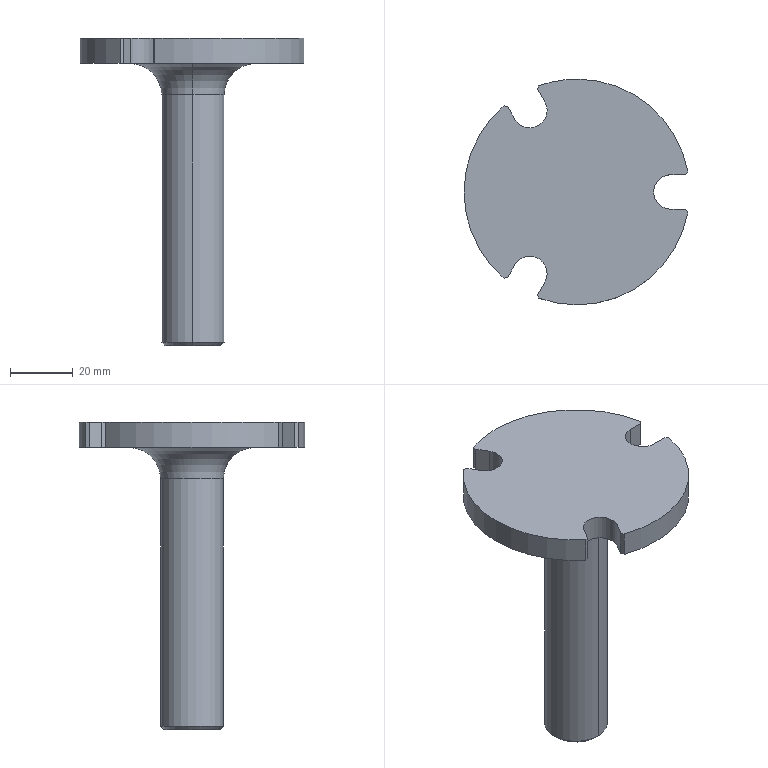NC program | NX | posted with a generic post | part box 71.434 x 72 x 98 mm
Lines 1 to 922 of 11060:
N10 G17 G21 G94 G90
(ZLEVEL_PROFILE_COPY_1 , TOOL : D6C)
N12 T06 M6
N14 G54
N16 G17 G0 G90 X-25.933 Y32.567 S5000 M3
N18 G43 Z30. H6
N20 Z-0.05
N22 G94 G1 X-25.748 Y31.712 F1800.
N24 G3 X-25.344 Y31.268 R0.6
N26 G1 X-22.161 Y30.416
N28 X-20.99 Y30.102
N30 G2 X-19.162 Y28.7 R3.01
N32 G1 X-16.874 Y24.736
N34 G3 X-13.472 Y23.824 R2.49
N36 X-12.561 Y27.226 R2.49
N38 G1 X-14.849 Y31.19
N40 G2 X-15.074 Y33.718 R3.01
N42 G1 X-15.079 Y33.731
N44 X-15.031 Y33.919
N46 X-14.836 Y34.644
N48 X-14.763 Y34.88
N50 X-14.77 Y34.888
N52 X-13.984 Y37.824
N54 G3 X-14.139 Y38.404 R0.6
N56 G1 X-14.782 Y39.046
N58 G0 X-26.004 Y32.57 Z-0.1
N60 G1 X-25.769 Y31.692
N62 G3 X-25.344 Y31.268 R0.6
N64 G1 X-22.161 Y30.416
N66 X-20.99 Y30.102
N68 G2 X-19.162 Y28.7 R3.01
N70 G1 X-16.874 Y24.736
N72 G3 X-13.472 Y23.824 R2.49
N74 X-12.561 Y27.226 R2.49
N76 G1 X-14.849 Y31.19
N78 G2 X-15.074 Y33.718 R3.01
N80 G1 X-15.079 Y33.731
N82 X-15.031 Y33.919
N84 X-14.836 Y34.644
N86 X-14.763 Y34.88
N88 X-14.77 Y34.888
N90 X-13.984 Y37.824
N92 G3 X-14.139 Y38.404 R0.6
N94 G1 X-14.782 Y39.046
N96 G0 X-26.004 Y32.57 Z-0.15
N98 G1 X-25.769 Y31.692
N100 G3 X-25.344 Y31.268 R0.6
N102 G1 X-22.161 Y30.416
N104 X-20.99 Y30.102
N106 G2 X-19.162 Y28.7 R3.01
N108 G1 X-16.874 Y24.736
N110 G3 X-13.472 Y23.824 R2.49
N112 X-12.561 Y27.226 R2.49
N114 G1 X-14.849 Y31.19
N116 G2 X-15.074 Y33.718 R3.01
N118 G1 X-15.079 Y33.731
N120 X-15.031 Y33.919
N122 X-14.836 Y34.644
N124 X-14.763 Y34.88
N126 X-14.77 Y34.888
N128 X-13.984 Y37.824
N130 G3 X-14.139 Y38.404 R0.6
N132 G1 X-14.782 Y39.046
N134 G0 X-26.004 Y32.57 Z-0.2
N136 G1 X-25.769 Y31.692
N138 G3 X-25.344 Y31.268 R0.6
N140 G1 X-22.161 Y30.416
N142 X-20.99 Y30.102
N144 G2 X-19.162 Y28.7 R3.01
N146 G1 X-16.874 Y24.736
N148 G3 X-13.472 Y23.824 R2.49
N150 X-12.561 Y27.226 R2.49
N152 G1 X-14.849 Y31.19
N154 G2 X-15.074 Y33.718 R3.01
N156 G1 X-15.079 Y33.731
N158 X-15.031 Y33.919
N160 X-14.836 Y34.644
N162 X-14.763 Y34.88
N164 X-14.77 Y34.888
N166 X-13.984 Y37.824
N168 G3 X-14.139 Y38.404 R0.6
N170 G1 X-14.782 Y39.046
N172 G0 X-26.004 Y32.57 Z-0.25
N174 G1 X-25.769 Y31.692
N176 G3 X-25.344 Y31.268 R0.6
N178 G1 X-22.161 Y30.416
N180 X-20.99 Y30.102
N182 G2 X-19.162 Y28.7 R3.01
N184 G1 X-16.874 Y24.736
N186 G3 X-13.472 Y23.824 R2.49
N188 X-12.561 Y27.226 R2.49
N190 G1 X-14.849 Y31.19
N192 G2 X-15.074 Y33.718 R3.01
N194 G1 X-15.079 Y33.731
N196 X-15.031 Y33.919
N198 X-14.836 Y34.645
N200 X-14.763 Y34.88
N202 X-14.77 Y34.888
N204 X-13.984 Y37.824
N206 G3 X-14.139 Y38.404 R0.6
N208 G1 X-14.782 Y39.046
N210 G0 X-26.004 Y32.57 Z-0.3
N212 G1 X-25.769 Y31.692
N214 G3 X-25.344 Y31.268 R0.6
N216 G1 X-22.161 Y30.416
N218 X-20.99 Y30.102
N220 G2 X-19.162 Y28.7 R3.01
N222 G1 X-16.874 Y24.736
N224 G3 X-13.472 Y23.824 R2.49
N226 X-12.561 Y27.226 R2.49
N228 G1 X-14.849 Y31.19
N230 G2 X-15.074 Y33.718 R3.01
N232 G1 X-15.079 Y33.731
N234 X-15.031 Y33.919
N236 X-14.836 Y34.645
N238 X-14.763 Y34.88
N240 X-14.77 Y34.888
N242 X-13.984 Y37.824
N244 G3 X-14.139 Y38.404 R0.6
N246 G1 X-14.782 Y39.046
N248 G0 X-26.004 Y32.57 Z-0.35
N250 G1 X-25.769 Y31.692
N252 G3 X-25.344 Y31.268 R0.6
N254 G1 X-22.161 Y30.416
N256 X-20.99 Y30.102
N258 G2 X-19.162 Y28.7 R3.01
N260 G1 X-16.874 Y24.736
N262 G3 X-13.472 Y23.824 R2.49
N264 X-12.561 Y27.226 R2.49
N266 G1 X-14.849 Y31.19
N268 G2 X-15.074 Y33.718 R3.01
N270 G1 X-15.079 Y33.731
N272 X-15.031 Y33.919
N274 X-14.836 Y34.645
N276 X-14.763 Y34.88
N278 X-14.77 Y34.888
N280 X-13.984 Y37.824
N282 G3 X-14.139 Y38.404 R0.6
N284 G1 X-14.782 Y39.046
N286 G0 X-26.004 Y32.57 Z-0.4
N288 G1 X-25.769 Y31.692
N290 G3 X-25.344 Y31.268 R0.6
N292 G1 X-22.161 Y30.416
N294 X-20.99 Y30.102
N296 G2 X-19.162 Y28.7 R3.01
N298 G1 X-16.874 Y24.736
N300 G3 X-13.472 Y23.824 R2.49
N302 X-12.561 Y27.226 R2.49
N304 G1 X-14.849 Y31.19
N306 G2 X-15.074 Y33.718 R3.01
N308 G1 X-15.079 Y33.731
N310 X-15.031 Y33.919
N312 X-14.836 Y34.645
N314 X-14.763 Y34.88
N316 X-14.77 Y34.888
N318 X-13.984 Y37.824
N320 G3 X-14.139 Y38.404 R0.6
N322 G1 X-14.782 Y39.046
N324 G0 X-26.004 Y32.57 Z-0.45
N326 G1 X-25.769 Y31.692
N328 G3 X-25.344 Y31.268 R0.6
N330 G1 X-22.161 Y30.416
N332 X-20.99 Y30.102
N334 G2 X-19.162 Y28.7 R3.01
N336 G1 X-16.874 Y24.736
N338 G3 X-13.472 Y23.824 R2.49
N340 X-12.561 Y27.226 R2.49
N342 G1 X-14.849 Y31.19
N344 G2 X-15.074 Y33.718 R3.01
N346 G1 X-15.079 Y33.731
N348 X-15.031 Y33.919
N350 X-14.836 Y34.645
N352 X-14.763 Y34.88
N354 X-14.77 Y34.888
N356 X-13.984 Y37.824
N358 G3 X-14.139 Y38.404 R0.6
N360 G1 X-14.782 Y39.046
N362 G0 X-26.004 Y32.57 Z-0.5
N364 G1 X-25.769 Y31.692
N366 G3 X-25.344 Y31.268 R0.6
N368 G1 X-22.161 Y30.416
N370 X-20.99 Y30.102
N372 G2 X-19.162 Y28.7 R3.01
N374 G1 X-16.874 Y24.736
N376 G3 X-13.472 Y23.824 R2.49
N378 X-12.561 Y27.226 R2.49
N380 G1 X-14.849 Y31.19
N382 G2 X-15.074 Y33.718 R3.01
N384 G1 X-15.079 Y33.731
N386 X-15.031 Y33.919
N388 X-14.836 Y34.645
N390 X-14.763 Y34.88
N392 X-14.77 Y34.888
N394 X-13.984 Y37.824
N396 G3 X-14.139 Y38.404 R0.6
N398 G1 X-14.782 Y39.046
N400 G0 X-26.004 Y32.57 Z-0.55
N402 G1 X-25.769 Y31.692
N404 G3 X-25.344 Y31.268 R0.6
N406 G1 X-22.161 Y30.416
N408 X-20.99 Y30.102
N410 G2 X-19.162 Y28.7 R3.01
N412 G1 X-16.874 Y24.736
N414 G3 X-13.472 Y23.824 R2.49
N416 X-12.561 Y27.226 R2.49
N418 G1 X-14.849 Y31.19
N420 G2 X-15.074 Y33.718 R3.01
N422 G1 X-15.079 Y33.731
N424 X-15.031 Y33.919
N426 X-14.836 Y34.645
N428 X-14.763 Y34.88
N430 X-14.77 Y34.888
N432 X-13.984 Y37.824
N434 G3 X-14.139 Y38.404 R0.6
N436 G1 X-14.782 Y39.046
N438 G0 X-26.004 Y32.57 Z-0.6
N440 G1 X-25.769 Y31.692
N442 G3 X-25.344 Y31.268 R0.6
N444 G1 X-22.161 Y30.416
N446 X-20.99 Y30.102
N448 G2 X-19.162 Y28.7 R3.01
N450 G1 X-16.874 Y24.736
N452 G3 X-13.472 Y23.824 R2.49
N454 X-12.561 Y27.226 R2.49
N456 G1 X-14.849 Y31.19
N458 G2 X-15.074 Y33.718 R3.01
N460 G1 X-15.079 Y33.731
N462 X-15.031 Y33.919
N464 X-14.836 Y34.645
N466 X-14.763 Y34.88
N468 X-14.77 Y34.888
N470 X-13.984 Y37.824
N472 G3 X-14.139 Y38.404 R0.6
N474 G1 X-14.782 Y39.046
N476 G0 X-26.004 Y32.57 Z-0.65
N478 G1 X-25.769 Y31.692
N480 G3 X-25.344 Y31.268 R0.6
N482 G1 X-22.161 Y30.416
N484 X-20.99 Y30.102
N486 G2 X-19.162 Y28.7 R3.01
N488 G1 X-16.874 Y24.736
N490 G3 X-13.472 Y23.824 R2.49
N492 X-12.561 Y27.226 R2.49
N494 G1 X-14.849 Y31.19
N496 G2 X-15.074 Y33.718 R3.01
N498 G1 X-15.079 Y33.731
N500 X-15.031 Y33.919
N502 X-14.836 Y34.645
N504 X-14.763 Y34.88
N506 X-14.77 Y34.888
N508 X-13.984 Y37.824
N510 G3 X-14.139 Y38.404 R0.6
N512 G1 X-14.782 Y39.046
N514 G0 X-26.004 Y32.57 Z-0.7
N516 G1 X-25.769 Y31.692
N518 G3 X-25.344 Y31.268 R0.6
N520 G1 X-22.161 Y30.416
N522 X-20.99 Y30.102
N524 G2 X-19.162 Y28.7 R3.01
N526 G1 X-16.874 Y24.736
N528 G3 X-13.472 Y23.824 R2.49
N530 X-12.561 Y27.226 R2.49
N532 G1 X-14.849 Y31.19
N534 G2 X-15.074 Y33.718 R3.01
N536 G1 X-15.079 Y33.731
N538 X-15.031 Y33.919
N540 X-14.836 Y34.645
N542 X-14.763 Y34.88
N544 X-14.77 Y34.888
N546 X-13.984 Y37.824
N548 G3 X-14.139 Y38.404 R0.6
N550 G1 X-14.782 Y39.046
N552 G0 X-26.004 Y32.57 Z-0.75
N554 G1 X-25.769 Y31.692
N556 G3 X-25.344 Y31.268 R0.6
N558 G1 X-22.161 Y30.416
N560 X-20.99 Y30.102
N562 G2 X-19.162 Y28.7 R3.01
N564 G1 X-16.874 Y24.736
N566 G3 X-13.472 Y23.824 R2.49
N568 X-12.561 Y27.226 R2.49
N570 G1 X-14.849 Y31.19
N572 G2 X-15.074 Y33.718 R3.01
N574 G1 X-15.079 Y33.731
N576 X-15.031 Y33.919
N578 X-14.836 Y34.645
N580 X-14.763 Y34.88
N582 X-14.77 Y34.888
N584 X-13.984 Y37.824
N586 G3 X-14.139 Y38.404 R0.6
N588 G1 X-14.782 Y39.046
N590 G0 X-26.004 Y32.57 Z-0.8
N592 G1 X-25.769 Y31.693
N594 G3 X-25.344 Y31.268 R0.6
N596 G1 X-22.161 Y30.416
N598 X-20.99 Y30.102
N600 G2 X-19.162 Y28.7 R3.01
N602 G1 X-16.874 Y24.736
N604 G3 X-13.472 Y23.824 R2.49
N606 X-12.561 Y27.226 R2.49
N608 G1 X-14.849 Y31.19
N610 G2 X-15.074 Y33.718 R3.01
N612 G1 X-15.079 Y33.731
N614 X-15.031 Y33.919
N616 X-14.836 Y34.645
N618 X-14.763 Y34.88
N620 X-14.77 Y34.888
N622 X-13.984 Y37.824
N624 G3 X-14.139 Y38.404 R0.6
N626 G1 X-14.782 Y39.046
N628 G0 X-26.004 Y32.57 Z-0.85
N630 G1 X-25.769 Y31.693
N632 G3 X-25.344 Y31.268 R0.6
N634 G1 X-22.161 Y30.416
N636 X-20.99 Y30.102
N638 G2 X-19.162 Y28.7 R3.01
N640 G1 X-16.874 Y24.736
N642 G3 X-13.472 Y23.824 R2.49
N644 X-12.561 Y27.226 R2.49
N646 G1 X-14.849 Y31.19
N648 G2 X-15.074 Y33.718 R3.01
N650 G1 X-15.08 Y33.731
N652 X-15.031 Y33.919
N654 X-14.836 Y34.645
N656 X-14.763 Y34.88
N658 X-14.77 Y34.888
N660 X-13.984 Y37.824
N662 G3 X-14.139 Y38.404 R0.6
N664 G1 X-14.782 Y39.046
N666 G0 X-26.004 Y32.57 Z-0.9
N668 G1 X-25.769 Y31.693
N670 G3 X-25.344 Y31.268 R0.6
N672 G1 X-22.161 Y30.416
N674 X-20.99 Y30.102
N676 G2 X-19.162 Y28.7 R3.01
N678 G1 X-16.874 Y24.736
N680 G3 X-13.472 Y23.824 R2.49
N682 X-12.561 Y27.226 R2.49
N684 G1 X-14.849 Y31.19
N686 G2 X-15.074 Y33.718 R3.01
N688 G1 X-15.08 Y33.731
N690 X-15.031 Y33.919
N692 X-14.836 Y34.645
N694 X-14.763 Y34.88
N696 X-14.77 Y34.888
N698 X-13.984 Y37.824
N700 G3 X-14.139 Y38.404 R0.6
N702 G1 X-14.782 Y39.046
N704 G0 X-26.004 Y32.57 Z-0.95
N706 G1 X-25.769 Y31.693
N708 G3 X-25.344 Y31.268 R0.6
N710 G1 X-22.161 Y30.416
N712 X-20.99 Y30.102
N714 G2 X-19.162 Y28.7 R3.01
N716 G1 X-16.874 Y24.736
N718 G3 X-13.472 Y23.824 R2.49
N720 X-12.561 Y27.226 R2.49
N722 G1 X-14.849 Y31.19
N724 G2 X-15.074 Y33.718 R3.01
N726 G1 X-15.08 Y33.731
N728 X-15.031 Y33.919
N730 X-14.836 Y34.645
N732 X-14.763 Y34.88
N734 X-14.77 Y34.888
N736 X-13.984 Y37.824
N738 G3 X-14.139 Y38.404 R0.6
N740 G1 X-14.782 Y39.046
N742 G0 X-26.004 Y32.57 Z-1.
N744 G1 X-25.769 Y31.693
N746 G3 X-25.344 Y31.268 R0.6
N748 G1 X-22.161 Y30.416
N750 X-20.99 Y30.102
N752 G2 X-19.162 Y28.7 R3.01
N754 G1 X-16.874 Y24.736
N756 G3 X-13.472 Y23.824 R2.49
N758 X-12.561 Y27.226 R2.49
N760 G1 X-14.849 Y31.19
N762 G2 X-15.074 Y33.718 R3.01
N764 G1 X-15.08 Y33.731
N766 X-15.031 Y33.919
N768 X-14.836 Y34.645
N770 X-14.763 Y34.88
N772 X-14.77 Y34.888
N774 X-13.984 Y37.824
N776 G3 X-14.139 Y38.404 R0.6
N778 G1 X-14.782 Y39.046
N780 G0 X-26.004 Y32.57 Z-1.05
N782 G1 X-25.769 Y31.693
N784 G3 X-25.344 Y31.268 R0.6
N786 G1 X-22.161 Y30.416
N788 X-20.99 Y30.102
N790 G2 X-19.162 Y28.7 R3.01
N792 G1 X-16.874 Y24.736
N794 G3 X-13.472 Y23.824 R2.49
N796 X-12.561 Y27.226 R2.49
N798 G1 X-14.849 Y31.19
N800 G2 X-15.074 Y33.718 R3.01
N802 G1 X-15.08 Y33.731
N804 X-15.031 Y33.919
N806 X-14.836 Y34.645
N808 X-14.763 Y34.88
N810 X-14.77 Y34.888
N812 X-13.984 Y37.824
N814 G3 X-14.139 Y38.404 R0.6
N816 G1 X-14.782 Y39.046
N818 G0 X-26.004 Y32.57 Z-1.1
N820 G1 X-25.769 Y31.693
N822 G3 X-25.344 Y31.268 R0.6
N824 G1 X-22.161 Y30.416
N826 X-20.99 Y30.102
N828 G2 X-19.162 Y28.7 R3.01
N830 G1 X-16.874 Y24.736
N832 G3 X-13.472 Y23.824 R2.49
N834 X-12.561 Y27.226 R2.49
N836 G1 X-14.849 Y31.19
N838 G2 X-15.074 Y33.718 R3.01
N840 G1 X-15.08 Y33.731
N842 X-15.031 Y33.919
N844 X-14.836 Y34.645
N846 X-14.763 Y34.88
N848 X-14.77 Y34.888
N850 X-13.984 Y37.824
N852 G3 X-14.139 Y38.404 R0.6
N854 G1 X-14.782 Y39.046
N856 G0 X-26.004 Y32.57 Z-1.15
N858 G1 X-25.769 Y31.693
N860 G3 X-25.344 Y31.268 R0.6
N862 G1 X-22.161 Y30.416
N864 X-20.99 Y30.102
N866 G2 X-19.162 Y28.7 R3.01
N868 G1 X-16.874 Y24.736
N870 G3 X-13.472 Y23.824 R2.49
N872 X-12.561 Y27.226 R2.49
N874 G1 X-14.849 Y31.19
N876 G2 X-15.074 Y33.718 R3.01
N878 G1 X-15.08 Y33.731
N880 X-15.031 Y33.919
N882 X-14.836 Y34.645
N884 X-14.763 Y34.88
N886 X-14.77 Y34.888
N888 X-13.984 Y37.824
N890 G3 X-14.139 Y38.404 R0.6
N892 G1 X-14.782 Y39.046
N894 G0 X-26.004 Y32.57 Z-1.2
N896 G1 X-25.769 Y31.693
N898 G3 X-25.344 Y31.268 R0.6
N900 G1 X-22.161 Y30.416
N902 X-20.99 Y30.102
N904 G2 X-19.162 Y28.7 R3.01
N906 G1 X-16.874 Y24.736
N908 G3 X-13.472 Y23.824 R2.49
N910 X-12.561 Y27.226 R2.49
N912 G1 X-14.849 Y31.19
N914 G2 X-15.074 Y33.718 R3.01
N916 G1 X-15.08 Y33.731
N918 X-15.031 Y33.919
N920 X-14.836 Y34.645
N922 X-14.763 Y34.88
N924 X-14.77 Y34.888
N926 X-13.984 Y37.824
N928 G3 X-14.139 Y38.404 R0.6
N930 G1 X-14.782 Y39.046
N932 G0 X-26.004 Y32.57 Z-1.25
N934 G1 X-25.769 Y31.693
N936 G3 X-25.344 Y31.268 R0.6
N938 G1 X-22.161 Y30.416
N940 X-20.99 Y30.102
N942 G2 X-19.162 Y28.7 R3.01
N944 G1 X-16.874 Y24.736
N946 G3 X-13.472 Y23.824 R2.49
N948 X-12.561 Y27.226 R2.49
N950 G1 X-14.849 Y31.19
N952 G2 X-15.074 Y33.718 R3.01
N954 G1 X-15.08 Y33.731
N956 X-15.031 Y33.919
N958 X-14.836 Y34.645
N960 X-14.763 Y34.88
N962 X-14.77 Y34.888
N964 X-13.984 Y37.824
N966 G3 X-14.139 Y38.404 R0.6
N968 G1 X-14.782 Y39.046
N970 G0 X-26.004 Y32.57 Z-1.3
N972 G1 X-25.769 Y31.693
N974 G3 X-25.344 Y31.268 R0.6
N976 G1 X-22.161 Y30.416
N978 X-20.99 Y30.102
N980 G2 X-19.162 Y28.7 R3.01
N982 G1 X-16.874 Y24.736
N984 G3 X-13.472 Y23.824 R2.49
N986 X-12.561 Y27.226 R2.49
N988 G1 X-14.849 Y31.19
N990 G2 X-15.074 Y33.718 R3.01
N992 G1 X-15.08 Y33.731
N994 X-15.031 Y33.919
N996 X-14.836 Y34.645
N998 X-14.763 Y34.88
N1000 X-14.77 Y34.888
N1002 X-13.984 Y37.824
N1004 G3 X-14.139 Y38.404 R0.6
N1006 G1 X-14.782 Y39.047
N1008 G0 X-26.004 Y32.57 Z-1.35
N1010 G1 X-25.769 Y31.693
N1012 G3 X-25.344 Y31.268 R0.6
N1014 G1 X-22.161 Y30.416
N1016 X-20.99 Y30.102
N1018 G2 X-19.162 Y28.7 R3.01
N1020 G1 X-16.874 Y24.736
N1022 G3 X-13.472 Y23.824 R2.49
N1024 X-12.561 Y27.226 R2.49
N1026 G1 X-14.849 Y31.19
N1028 G2 X-15.074 Y33.718 R3.01
N1030 G1 X-15.08 Y33.731
N1032 X-15.031 Y33.919
N1034 X-14.836 Y34.645
N1036 X-14.763 Y34.88
N1038 X-14.77 Y34.888
N1040 X-13.984 Y37.824
N1042 G3 X-14.139 Y38.404 R0.6
N1044 G1 X-14.782 Y39.047
N1046 G0 X-26.004 Y32.57 Z-1.4
N1048 G1 X-25.769 Y31.693
N1050 G3 X-25.344 Y31.268 R0.6
N1052 G1 X-22.161 Y30.416
N1054 X-20.99 Y30.102
N1056 G2 X-19.162 Y28.7 R3.01
N1058 G1 X-16.874 Y24.736
N1060 G3 X-13.472 Y23.824 R2.49
N1062 X-12.561 Y27.226 R2.49
N1064 G1 X-14.849 Y31.19
N1066 G2 X-15.074 Y33.718 R3.01
N1068 G1 X-15.08 Y33.731
N1070 X-15.031 Y33.919
N1072 X-14.836 Y34.645
N1074 X-14.763 Y34.88
N1076 X-14.77 Y34.888
N1078 X-13.984 Y37.824
N1080 G3 X-14.139 Y38.404 R0.6
N1082 G1 X-14.782 Y39.047
N1084 G0 X-26.004 Y32.57 Z-1.45
N1086 G1 X-25.769 Y31.693
N1088 G3 X-25.344 Y31.268 R0.6
N1090 G1 X-22.161 Y30.416
N1092 X-20.99 Y30.102
N1094 G2 X-19.162 Y28.7 R3.01
N1096 G1 X-16.874 Y24.736
N1098 G3 X-13.472 Y23.824 R2.49
N1100 X-12.561 Y27.226 R2.49
N1102 G1 X-14.849 Y31.19
N1104 G2 X-15.074 Y33.718 R3.01
N1106 G1 X-15.08 Y33.731
N1108 X-15.031 Y33.919
N1110 X-14.836 Y34.645
N1112 X-14.763 Y34.88
N1114 X-14.77 Y34.888
N1116 X-13.984 Y37.824
N1118 G3 X-14.139 Y38.404 R0.6
N1120 G1 X-14.782 Y39.047
N1122 G0 X-26.004 Y32.57 Z-1.5
N1124 G1 X-25.769 Y31.693
N1126 G3 X-25.344 Y31.268 R0.6
N1128 G1 X-22.161 Y30.416
N1130 X-20.99 Y30.102
N1132 G2 X-19.162 Y28.7 R3.01
N1134 G1 X-16.874 Y24.736
N1136 G3 X-13.472 Y23.824 R2.49
N1138 X-12.561 Y27.226 R2.49
N1140 G1 X-14.849 Y31.19
N1142 G2 X-15.074 Y33.718 R3.01
N1144 G1 X-15.08 Y33.731
N1146 X-15.031 Y33.919
N1148 X-14.836 Y34.645
N1150 X-14.763 Y34.88
N1152 X-14.77 Y34.888
N1154 X-13.984 Y37.824
N1156 G3 X-14.139 Y38.404 R0.6
N1158 G1 X-14.782 Y39.047
N1160 G0 X-26.004 Y32.57 Z-1.55
N1162 G1 X-25.769 Y31.693
N1164 G3 X-25.344 Y31.268 R0.6
N1166 G1 X-22.161 Y30.416
N1168 X-20.99 Y30.102
N1170 G2 X-19.162 Y28.7 R3.01
N1172 G1 X-16.874 Y24.736
N1174 G3 X-13.472 Y23.824 R2.49
N1176 X-12.561 Y27.226 R2.49
N1178 G1 X-14.849 Y31.19
N1180 G2 X-15.074 Y33.718 R3.01
N1182 G1 X-15.08 Y33.731
N1184 X-15.031 Y33.919
N1186 X-14.836 Y34.645
N1188 X-14.763 Y34.88
N1190 X-14.77 Y34.888
N1192 X-13.984 Y37.824
N1194 G3 X-14.139 Y38.404 R0.6
N1196 G1 X-14.782 Y39.047
N1198 G0 X-26.004 Y32.57 Z-1.6
N1200 G1 X-25.769 Y31.693
N1202 G3 X-25.344 Y31.268 R0.6
N1204 G1 X-22.161 Y30.416
N1206 X-20.99 Y30.102
N1208 G2 X-19.162 Y28.7 R3.01
N1210 G1 X-16.874 Y24.736
N1212 G3 X-13.472 Y23.824 R2.49
N1214 X-12.561 Y27.226 R2.49
N1216 G1 X-14.849 Y31.19
N1218 G2 X-15.074 Y33.718 R3.01
N1220 G1 X-15.08 Y33.731
N1222 X-15.031 Y33.919
N1224 X-14.836 Y34.645
N1226 X-14.763 Y34.88
N1228 X-14.77 Y34.888
N1230 X-13.984 Y37.824
N1232 G3 X-14.139 Y38.404 R0.6
N1234 G1 X-14.782 Y39.047
N1236 G0 X-26.004 Y32.57 Z-1.65
N1238 G1 X-25.769 Y31.693
N1240 G3 X-25.344 Y31.268 R0.6
N1242 G1 X-22.161 Y30.416
N1244 X-20.99 Y30.102
N1246 G2 X-19.162 Y28.7 R3.01
N1248 G1 X-16.874 Y24.736
N1250 G3 X-13.472 Y23.824 R2.49
N1252 X-12.561 Y27.226 R2.49
N1254 G1 X-14.849 Y31.19
N1256 G2 X-15.074 Y33.718 R3.01
N1258 G1 X-15.08 Y33.731
N1260 X-15.031 Y33.919
N1262 X-14.836 Y34.645
N1264 X-14.763 Y34.88
N1266 X-14.77 Y34.888
N1268 X-13.984 Y37.824
N1270 G3 X-14.139 Y38.404 R0.6
N1272 G1 X-14.782 Y39.047
N1274 G0 X-26.004 Y32.57 Z-1.7
N1276 G1 X-25.769 Y31.693
N1278 G3 X-25.344 Y31.268 R0.6
N1280 G1 X-22.161 Y30.416
N1282 X-20.99 Y30.102
N1284 G2 X-19.162 Y28.7 R3.01
N1286 G1 X-16.874 Y24.736
N1288 G3 X-13.472 Y23.824 R2.49
N1290 X-12.561 Y27.226 R2.49
N1292 G1 X-14.849 Y31.19
N1294 G2 X-15.074 Y33.718 R3.01
N1296 G1 X-15.08 Y33.731
N1298 X-15.031 Y33.919
N1300 X-14.836 Y34.645
N1302 X-14.763 Y34.88
N1304 X-14.77 Y34.888
N1306 X-13.984 Y37.824
N1308 G3 X-14.139 Y38.404 R0.6
N1310 G1 X-14.782 Y39.047
N1312 G0 X-26.004 Y32.57 Z-1.75
N1314 G1 X-25.769 Y31.693
N1316 G3 X-25.344 Y31.268 R0.6
N1318 G1 X-22.161 Y30.416
N1320 X-20.99 Y30.102
N1322 G2 X-19.162 Y28.7 R3.01
N1324 G1 X-16.874 Y24.736
N1326 G3 X-13.472 Y23.824 R2.49
N1328 X-12.561 Y27.226 R2.49
N1330 G1 X-14.849 Y31.19
N1332 G2 X-15.074 Y33.718 R3.01
N1334 G1 X-15.08 Y33.731
N1336 X-15.031 Y33.919
N1338 X-14.836 Y34.645
N1340 X-14.763 Y34.88
N1342 X-14.77 Y34.888
N1344 X-13.984 Y37.824
N1346 G3 X-14.139 Y38.404 R0.6
N1348 G1 X-14.782 Y39.047
N1350 G0 X-26.004 Y32.57 Z-1.8
N1352 G1 X-25.769 Y31.693
N1354 G3 X-25.344 Y31.268 R0.6
N1356 G1 X-22.161 Y30.416
N1358 X-20.99 Y30.102
N1360 G2 X-19.162 Y28.7 R3.01
N1362 G1 X-16.874 Y24.736
N1364 G3 X-13.472 Y23.824 R2.49
N1366 X-12.561 Y27.226 R2.49
N1368 G1 X-14.849 Y31.19
N1370 G2 X-15.074 Y33.718 R3.01
N1372 G1 X-15.08 Y33.731
N1374 X-15.031 Y33.919
N1376 X-14.836 Y34.645
N1378 X-14.763 Y34.88
N1380 X-14.77 Y34.888
N1382 X-13.984 Y37.824
N1384 G3 X-14.139 Y38.404 R0.6
N1386 G1 X-14.782 Y39.047
N1388 G0 X-26.004 Y32.57 Z-1.85
N1390 G1 X-25.769 Y31.693
N1392 G3 X-25.344 Y31.268 R0.6
N1394 G1 X-22.161 Y30.416
N1396 X-20.99 Y30.102
N1398 G2 X-19.162 Y28.7 R3.01
N1400 G1 X-16.874 Y24.736
N1402 G3 X-13.472 Y23.824 R2.49
N1404 X-12.561 Y27.226 R2.49
N1406 G1 X-14.849 Y31.19
N1408 G2 X-15.074 Y33.718 R3.01
N1410 G1 X-15.08 Y33.731
N1412 X-15.031 Y33.919
N1414 X-14.836 Y34.645
N1416 X-14.763 Y34.88
N1418 X-14.77 Y34.888
N1420 X-13.984 Y37.824
N1422 G3 X-14.139 Y38.404 R0.6
N1424 G1 X-14.782 Y39.047
N1426 G0 X-26.004 Y32.57 Z-1.9
N1428 G1 X-25.769 Y31.693
N1430 G3 X-25.344 Y31.268 R0.6
N1432 G1 X-22.161 Y30.416
N1434 X-20.99 Y30.102
N1436 G2 X-19.162 Y28.7 R3.01
N1438 G1 X-16.874 Y24.736
N1440 G3 X-13.472 Y23.824 R2.49
N1442 X-12.561 Y27.226 R2.49
N1444 G1 X-14.849 Y31.19
N1446 G2 X-15.074 Y33.718 R3.01
N1448 G1 X-15.08 Y33.731
N1450 X-15.031 Y33.919
N1452 X-14.836 Y34.645
N1454 X-14.763 Y34.88
N1456 X-14.77 Y34.888
N1458 X-13.984 Y37.824
N1460 G3 X-14.139 Y38.404 R0.6
N1462 G1 X-14.782 Y39.047
N1464 G0 X-26.004 Y32.57 Z-1.95
N1466 G1 X-25.769 Y31.693
N1468 G3 X-25.344 Y31.268 R0.6
N1470 G1 X-22.161 Y30.416
N1472 X-20.99 Y30.102
N1474 G2 X-19.162 Y28.7 R3.01
N1476 G1 X-16.874 Y24.736
N1478 G3 X-13.472 Y23.824 R2.49
N1480 X-12.561 Y27.226 R2.49
N1482 G1 X-14.849 Y31.19
N1484 G2 X-15.074 Y33.718 R3.01
N1486 G1 X-15.08 Y33.731
N1488 X-15.031 Y33.919
N1490 X-14.836 Y34.645
N1492 X-14.763 Y34.88
N1494 X-14.77 Y34.888
N1496 X-13.984 Y37.824
N1498 G3 X-14.139 Y38.404 R0.6
N1500 G1 X-14.782 Y39.047
N1502 G0 X-26.004 Y32.57 Z-2.
N1504 G1 X-25.769 Y31.693
N1506 G3 X-25.344 Y31.268 R0.6
N1508 G1 X-22.161 Y30.416
N1510 X-20.99 Y30.102
N1512 G2 X-19.162 Y28.7 R3.01
N1514 G1 X-16.874 Y24.736
N1516 G3 X-13.472 Y23.824 R2.49
N1518 X-12.561 Y27.226 R2.49
N1520 G1 X-14.849 Y31.19
N1522 G2 X-15.074 Y33.718 R3.01
N1524 G1 X-15.08 Y33.731
N1526 X-15.031 Y33.919
N1528 X-14.836 Y34.645
N1530 X-14.763 Y34.88
N1532 X-14.77 Y34.888
N1534 X-13.984 Y37.824
N1536 G3 X-14.139 Y38.404 R0.6
N1538 G1 X-14.782 Y39.047
N1540 G0 X-26.004 Y32.57 Z-2.05
N1542 G1 X-25.769 Y31.693
N1544 G3 X-25.344 Y31.268 R0.6
N1546 G1 X-22.161 Y30.416
N1548 X-20.99 Y30.102
N1550 G2 X-19.162 Y28.7 R3.01
N1552 G1 X-16.874 Y24.736
N1554 G3 X-13.472 Y23.824 R2.49
N1556 X-12.561 Y27.226 R2.49
N1558 G1 X-14.849 Y31.19
N1560 G2 X-15.074 Y33.718 R3.01
N1562 G1 X-15.08 Y33.731
N1564 X-15.031 Y33.919
N1566 X-14.836 Y34.645
N1568 X-14.763 Y34.88
N1570 X-14.77 Y34.888
N1572 X-13.984 Y37.824
N1574 G3 X-14.139 Y38.404 R0.6
N1576 G1 X-14.782 Y39.047
N1578 G0 X-26.004 Y32.57 Z-2.1
N1580 G1 X-25.769 Y31.693
N1582 G3 X-25.344 Y31.268 R0.6
N1584 G1 X-22.161 Y30.416
N1586 X-20.99 Y30.102
N1588 G2 X-19.162 Y28.7 R3.01
N1590 G1 X-16.874 Y24.736
N1592 G3 X-13.472 Y23.824 R2.49
N1594 X-12.561 Y27.226 R2.49
N1596 G1 X-14.849 Y31.19
N1598 G2 X-15.074 Y33.718 R3.01
N1600 G1 X-15.08 Y33.731
N1602 X-15.031 Y33.919
N1604 X-14.836 Y34.645
N1606 X-14.763 Y34.88
N1608 X-14.77 Y34.888
N1610 X-13.984 Y37.824
N1612 G3 X-14.139 Y38.404 R0.6
N1614 G1 X-14.782 Y39.047
N1616 G0 X-26.004 Y32.57 Z-2.15
N1618 G1 X-25.769 Y31.693
N1620 G3 X-25.344 Y31.268 R0.6
N1622 G1 X-22.161 Y30.416
N1624 X-20.99 Y30.102
N1626 G2 X-19.162 Y28.7 R3.01
N1628 G1 X-16.874 Y24.736
N1630 G3 X-13.472 Y23.824 R2.49
N1632 X-12.561 Y27.226 R2.49
N1634 G1 X-14.849 Y31.19
N1636 G2 X-15.074 Y33.718 R3.01
N1638 G1 X-15.08 Y33.731
N1640 X-15.031 Y33.919
N1642 X-14.836 Y34.645
N1644 X-14.763 Y34.88
N1646 X-14.77 Y34.888
N1648 X-13.984 Y37.824
N1650 G3 X-14.139 Y38.404 R0.6
N1652 G1 X-14.782 Y39.047
N1654 G0 X-26.004 Y32.57 Z-2.2
N1656 G1 X-25.769 Y31.693
N1658 G3 X-25.344 Y31.268 R0.6
N1660 G1 X-22.161 Y30.416
N1662 X-20.99 Y30.102
N1664 G2 X-19.162 Y28.7 R3.01
N1666 G1 X-16.874 Y24.736
N1668 G3 X-13.472 Y23.824 R2.49
N1670 X-12.561 Y27.226 R2.49
N1672 G1 X-14.849 Y31.19
N1674 G2 X-15.074 Y33.718 R3.01
N1676 G1 X-15.08 Y33.731
N1678 X-15.031 Y33.919
N1680 X-14.836 Y34.645
N1682 X-14.763 Y34.88
N1684 X-14.77 Y34.888
N1686 X-13.984 Y37.824
N1688 G3 X-14.139 Y38.404 R0.6
N1690 G1 X-14.782 Y39.047
N1692 G0 X-26.004 Y32.57 Z-2.25
N1694 G1 X-25.769 Y31.693
N1696 G3 X-25.344 Y31.268 R0.6
N1698 G1 X-22.161 Y30.416
N1700 X-20.99 Y30.102
N1702 G2 X-19.162 Y28.7 R3.01
N1704 G1 X-16.874 Y24.736
N1706 G3 X-13.472 Y23.824 R2.49
N1708 X-12.561 Y27.226 R2.49
N1710 G1 X-14.849 Y31.19
N1712 G2 X-15.074 Y33.718 R3.01
N1714 G1 X-15.08 Y33.731
N1716 X-15.031 Y33.919
N1718 X-14.836 Y34.645
N1720 X-14.763 Y34.88
N1722 X-14.77 Y34.888
N1724 X-13.984 Y37.824
N1726 G3 X-14.139 Y38.404 R0.6
N1728 G1 X-14.782 Y39.047
N1730 G0 X-26.004 Y32.57 Z-2.3
N1732 G1 X-25.768 Y31.693
N1734 G3 X-25.344 Y31.268 R0.6
N1736 G1 X-22.161 Y30.416
N1738 X-20.99 Y30.102
N1740 G2 X-19.162 Y28.7 R3.01
N1742 G1 X-16.874 Y24.736
N1744 G3 X-13.472 Y23.824 R2.49
N1746 X-12.561 Y27.226 R2.49
N1748 G1 X-14.849 Y31.19
N1750 G2 X-15.074 Y33.718 R3.01
N1752 G1 X-15.08 Y33.731
N1754 X-15.031 Y33.919
N1756 X-14.836 Y34.645
N1758 X-14.763 Y34.88
N1760 X-14.77 Y34.888
N1762 X-13.984 Y37.824
N1764 G3 X-14.139 Y38.404 R0.6
N1766 G1 X-14.782 Y39.047
N1768 G0 X-26.004 Y32.57 Z-2.35
N1770 G1 X-25.768 Y31.693
N1772 G3 X-25.344 Y31.268 R0.6
N1774 G1 X-22.161 Y30.416
N1776 X-20.99 Y30.102
N1778 G2 X-19.162 Y28.7 R3.01
N1780 G1 X-16.874 Y24.736
N1782 G3 X-13.472 Y23.824 R2.49
N1784 X-12.561 Y27.226 R2.49
N1786 G1 X-14.849 Y31.19
N1788 G2 X-15.074 Y33.718 R3.01
N1790 G1 X-15.08 Y33.731
N1792 X-15.031 Y33.919
N1794 X-14.836 Y34.645
N1796 X-14.763 Y34.88
N1798 X-14.77 Y34.888
N1800 X-13.984 Y37.824
N1802 G3 X-14.139 Y38.404 R0.6
N1804 G1 X-14.782 Y39.047
N1806 G0 X-26.004 Y32.57 Z-2.4
N1808 G1 X-25.768 Y31.693
N1810 G3 X-25.344 Y31.268 R0.6
N1812 G1 X-22.161 Y30.416
N1814 X-20.99 Y30.102
N1816 G2 X-19.162 Y28.7 R3.01
N1818 G1 X-16.874 Y24.736
N1820 G3 X-13.472 Y23.824 R2.49
N1822 X-12.561 Y27.226 R2.49
N1824 G1 X-14.849 Y31.19
N1826 G2 X-15.074 Y33.718 R3.01
N1828 G1 X-15.08 Y33.731
N1830 X-15.031 Y33.919
N1832 X-14.836 Y34.645
N1834 X-14.763 Y34.88
N1836 X-14.77 Y34.888
N1838 X-13.984 Y37.824
N1840 G3 X-14.139 Y38.404 R0.6
N1842 G1 X-14.782 Y39.047